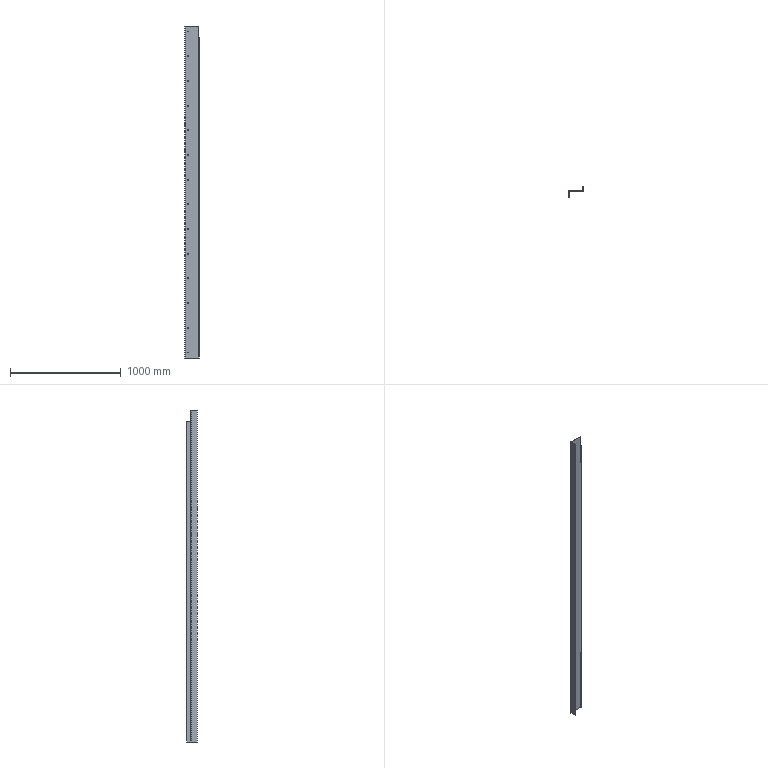Part | STEP file | TS-Z001-06 | 1 solid | 52 faces | box 131 x 95 x 2995 mm | volume 1974273 mm3 | cylinder 32 | plane 20 | commonest cylinder face diameters 8 x28 0.4 x2 6.4 x2